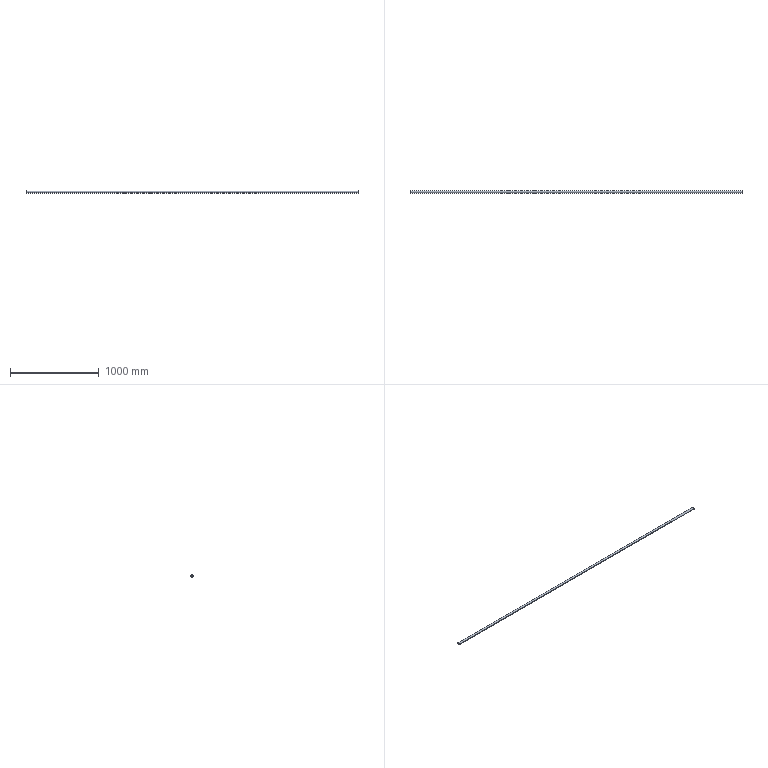Part | STEP file | 粉仓护栏栏杆2_Default<As Machined> | 1 solid | 6 faces | box 3734 x 25 x 25 mm | volume 413507 mm3 | cylinder 4 | plane 2 | commonest cylinder face diameters 22 x2 25 x2
STEP:
#1=CARTESIAN_POINT('',(0.,0.,0.));
#2=DIRECTION('',(0.,0.,1.));
#3=DIRECTION('',(1.,0.,0.));
#4=AXIS2_PLACEMENT_3D('',#1,#2,#3);
#5=CARTESIAN_POINT('',(1867.,12.5,0.));
#6=VERTEX_POINT('',#5);
#7=CARTESIAN_POINT('',(1867.,-12.5,0.));
#8=VERTEX_POINT('',#7);
#9=CARTESIAN_POINT('',(1867.,0.,0.));
#10=DIRECTION('',(1.,0.,0.));
#11=DIRECTION('',(0.,1.,0.));
#12=AXIS2_PLACEMENT_3D('',#9,#10,#11);
#13=CIRCLE('',#12,12.5);
#14=CARTESIAN_POINT('',(1867.,0.,0.));
#15=DIRECTION('',(-1.,0.,0.));
#16=DIRECTION('',(0.,-1.,0.));
#17=AXIS2_PLACEMENT_3D('',#14,#15,#16);
#18=CYLINDRICAL_SURFACE('',#17,12.5);
#19=CARTESIAN_POINT('',(3.142,0.));
#20=DIRECTION('',(-1.,0.));
#21=VECTOR('',#20,1.);
#22=LINE('',#19,#21);
#23=(GEOMETRIC_REPRESENTATION_CONTEXT(2)PARAMETRIC_REPRESENTATION_CONTEXT()REPRESENTATION_CONTEXT('',''));
#24=DEFINITIONAL_REPRESENTATION('',(#22),#23);
#25=PCURVE('',#18,#24);
#26=CARTESIAN_POINT('',(1867.,0.,0.));
#27=DIRECTION('',(1.,0.,0.));
#28=DIRECTION('',(0.,1.,0.));
#29=AXIS2_PLACEMENT_3D('',#26,#27,#28);
#30=PLANE('',#29);
#31=CARTESIAN_POINT('',(0.,0.));
#32=DIRECTION('',(1.,0.));
#33=AXIS2_PLACEMENT_2D('',#31,#32);
#34=CIRCLE('',#33,12.5);
#35=(GEOMETRIC_REPRESENTATION_CONTEXT(2)PARAMETRIC_REPRESENTATION_CONTEXT()REPRESENTATION_CONTEXT('',''));
#36=DEFINITIONAL_REPRESENTATION('',(#34),#35);
#37=PCURVE('',#30,#36);
#38=SURFACE_CURVE('',#13,(#25,#37),.PCURVE_S1.);
#39=EDGE_CURVE('',#6,#8,#38,.T.);
#40=ORIENTED_EDGE('',*,*,#39,.F.);
#41=CARTESIAN_POINT('',(-1867.,12.5,0.));
#42=VERTEX_POINT('',#41);
#43=CARTESIAN_POINT('',(1867.,12.5,0.));
#44=DIRECTION('',(-1.,0.,0.));
#45=VECTOR('',#44,1.);
#46=LINE('',#43,#45);
#47=CARTESIAN_POINT('',(3.142,0.));
#48=DIRECTION('',(0.,1.));
#49=VECTOR('',#48,1.);
#50=LINE('',#47,#49);
#51=(GEOMETRIC_REPRESENTATION_CONTEXT(2)PARAMETRIC_REPRESENTATION_CONTEXT()REPRESENTATION_CONTEXT('',''));
#52=DEFINITIONAL_REPRESENTATION('',(#50),#51);
#53=PCURVE('',#18,#52);
#54=CARTESIAN_POINT('',(1867.,0.,0.));
#55=DIRECTION('',(-1.,0.,0.));
#56=DIRECTION('',(0.,-1.,0.));
#57=AXIS2_PLACEMENT_3D('',#54,#55,#56);
#58=CYLINDRICAL_SURFACE('',#57,12.5);
#59=CARTESIAN_POINT('',(3.142,0.));
#60=DIRECTION('',(0.,1.));
#61=VECTOR('',#60,1.);
#62=LINE('',#59,#61);
#63=(GEOMETRIC_REPRESENTATION_CONTEXT(2)PARAMETRIC_REPRESENTATION_CONTEXT()REPRESENTATION_CONTEXT('',''));
#64=DEFINITIONAL_REPRESENTATION('',(#62),#63);
#65=PCURVE('',#58,#64);
#66=SURFACE_CURVE('',#46,(#53,#65),.PCURVE_S1.);
#67=EDGE_CURVE('',#6,#42,#66,.T.);
#68=ORIENTED_EDGE('',*,*,#67,.T.);
#69=CARTESIAN_POINT('',(-1867.,-12.5,0.));
#70=VERTEX_POINT('',#69);
#71=CARTESIAN_POINT('',(-1867.,0.,0.));
#72=DIRECTION('',(1.,0.,0.));
#73=DIRECTION('',(0.,1.,0.));
#74=AXIS2_PLACEMENT_3D('',#71,#72,#73);
#75=CIRCLE('',#74,12.5);
#76=CARTESIAN_POINT('',(3.142,3734.));
#77=DIRECTION('',(-1.,0.));
#78=VECTOR('',#77,1.);
#79=LINE('',#76,#78);
#80=(GEOMETRIC_REPRESENTATION_CONTEXT(2)PARAMETRIC_REPRESENTATION_CONTEXT()REPRESENTATION_CONTEXT('',''));
#81=DEFINITIONAL_REPRESENTATION('',(#79),#80);
#82=PCURVE('',#18,#81);
#83=CARTESIAN_POINT('',(-1867.,0.,0.));
#84=DIRECTION('',(1.,0.,0.));
#85=DIRECTION('',(0.,1.,0.));
#86=AXIS2_PLACEMENT_3D('',#83,#84,#85);
#87=PLANE('',#86);
#88=CARTESIAN_POINT('',(0.,0.));
#89=DIRECTION('',(1.,0.));
#90=AXIS2_PLACEMENT_2D('',#88,#89);
#91=CIRCLE('',#90,12.5);
#92=(GEOMETRIC_REPRESENTATION_CONTEXT(2)PARAMETRIC_REPRESENTATION_CONTEXT()REPRESENTATION_CONTEXT('',''));
#93=DEFINITIONAL_REPRESENTATION('',(#91),#92);
#94=PCURVE('',#87,#93);
#95=SURFACE_CURVE('',#75,(#82,#94),.PCURVE_S1.);
#96=EDGE_CURVE('',#42,#70,#95,.T.);
#97=ORIENTED_EDGE('',*,*,#96,.T.);
#98=CARTESIAN_POINT('',(1867.,-12.5,0.));
#99=DIRECTION('',(-1.,0.,0.));
#100=VECTOR('',#99,1.);
#101=LINE('',#98,#100);
#102=CARTESIAN_POINT('',(0.,0.));
#103=DIRECTION('',(0.,1.));
#104=VECTOR('',#103,1.);
#105=LINE('',#102,#104);
#106=(GEOMETRIC_REPRESENTATION_CONTEXT(2)PARAMETRIC_REPRESENTATION_CONTEXT()REPRESENTATION_CONTEXT('',''));
#107=DEFINITIONAL_REPRESENTATION('',(#105),#106);
#108=PCURVE('',#18,#107);
#109=CARTESIAN_POINT('',(6.283,0.));
#110=DIRECTION('',(0.,1.));
#111=VECTOR('',#110,1.);
#112=LINE('',#109,#111);
#113=(GEOMETRIC_REPRESENTATION_CONTEXT(2)PARAMETRIC_REPRESENTATION_CONTEXT()REPRESENTATION_CONTEXT('',''));
#114=DEFINITIONAL_REPRESENTATION('',(#112),#113);
#115=PCURVE('',#58,#114);
#116=SURFACE_CURVE('',#101,(#108,#115),.PCURVE_S1.);
#117=EDGE_CURVE('',#8,#70,#116,.T.);
#118=ORIENTED_EDGE('',*,*,#117,.F.);
#119=EDGE_LOOP('',(#40,#68,#97,#118));
#120=FACE_BOUND('',#119,.T.);
#121=ADVANCED_FACE('',(#120),#18,.T.);
#122=CARTESIAN_POINT('',(1867.,-11.,0.));
#123=VERTEX_POINT('',#122);
#124=CARTESIAN_POINT('',(-1867.,-11.,0.));
#125=VERTEX_POINT('',#124);
#126=CARTESIAN_POINT('',(1867.,-11.,0.));
#127=DIRECTION('',(-1.,0.,0.));
#128=VECTOR('',#127,1.);
#129=LINE('',#126,#128);
#130=CARTESIAN_POINT('',(1867.,0.,0.));
#131=DIRECTION('',(-1.,0.,0.));
#132=DIRECTION('',(0.,-1.,0.));
#133=AXIS2_PLACEMENT_3D('',#130,#131,#132);
#134=CYLINDRICAL_SURFACE('',#133,11.);
#135=CARTESIAN_POINT('',(6.283,0.));
#136=DIRECTION('',(0.,1.));
#137=VECTOR('',#136,1.);
#138=LINE('',#135,#137);
#139=(GEOMETRIC_REPRESENTATION_CONTEXT(2)PARAMETRIC_REPRESENTATION_CONTEXT()REPRESENTATION_CONTEXT('',''));
#140=DEFINITIONAL_REPRESENTATION('',(#138),#139);
#141=PCURVE('',#134,#140);
#142=CARTESIAN_POINT('',(1867.,0.,0.));
#143=DIRECTION('',(-1.,0.,0.));
#144=DIRECTION('',(0.,-1.,0.));
#145=AXIS2_PLACEMENT_3D('',#142,#143,#144);
#146=CYLINDRICAL_SURFACE('',#145,11.);
#147=CARTESIAN_POINT('',(0.,0.));
#148=DIRECTION('',(0.,1.));
#149=VECTOR('',#148,1.);
#150=LINE('',#147,#149);
#151=(GEOMETRIC_REPRESENTATION_CONTEXT(2)PARAMETRIC_REPRESENTATION_CONTEXT()REPRESENTATION_CONTEXT('',''));
#152=DEFINITIONAL_REPRESENTATION('',(#150),#151);
#153=PCURVE('',#146,#152);
#154=SURFACE_CURVE('',#129,(#141,#153),.PCURVE_S1.);
#155=EDGE_CURVE('',#123,#125,#154,.T.);
#156=ORIENTED_EDGE('',*,*,#155,.T.);
#157=CARTESIAN_POINT('',(-1867.,11.,0.));
#158=VERTEX_POINT('',#157);
#159=CARTESIAN_POINT('',(-1867.,0.,0.));
#160=DIRECTION('',(1.,0.,0.));
#161=DIRECTION('',(0.,1.,0.));
#162=AXIS2_PLACEMENT_3D('',#159,#160,#161);
#163=CIRCLE('',#162,11.);
#164=CARTESIAN_POINT('',(9.425,3734.));
#165=DIRECTION('',(-1.,0.));
#166=VECTOR('',#165,1.);
#167=LINE('',#164,#166);
#168=(GEOMETRIC_REPRESENTATION_CONTEXT(2)PARAMETRIC_REPRESENTATION_CONTEXT()REPRESENTATION_CONTEXT('',''));
#169=DEFINITIONAL_REPRESENTATION('',(#167),#168);
#170=PCURVE('',#134,#169);
#171=CARTESIAN_POINT('',(0.,0.));
#172=DIRECTION('',(1.,0.));
#173=AXIS2_PLACEMENT_2D('',#171,#172);
#174=CIRCLE('',#173,11.);
#175=(GEOMETRIC_REPRESENTATION_CONTEXT(2)PARAMETRIC_REPRESENTATION_CONTEXT()REPRESENTATION_CONTEXT('',''));
#176=DEFINITIONAL_REPRESENTATION('',(#174),#175);
#177=PCURVE('',#87,#176);
#178=SURFACE_CURVE('',#163,(#170,#177),.PCURVE_S1.);
#179=EDGE_CURVE('',#125,#158,#178,.T.);
#180=ORIENTED_EDGE('',*,*,#179,.T.);
#181=CARTESIAN_POINT('',(1867.,11.,0.));
#182=VERTEX_POINT('',#181);
#183=CARTESIAN_POINT('',(1867.,11.,0.));
#184=DIRECTION('',(-1.,0.,0.));
#185=VECTOR('',#184,1.);
#186=LINE('',#183,#185);
#187=CARTESIAN_POINT('',(3.142,0.));
#188=DIRECTION('',(0.,1.));
#189=VECTOR('',#188,1.);
#190=LINE('',#187,#189);
#191=(GEOMETRIC_REPRESENTATION_CONTEXT(2)PARAMETRIC_REPRESENTATION_CONTEXT()REPRESENTATION_CONTEXT('',''));
#192=DEFINITIONAL_REPRESENTATION('',(#190),#191);
#193=PCURVE('',#134,#192);
#194=CARTESIAN_POINT('',(3.142,0.));
#195=DIRECTION('',(0.,1.));
#196=VECTOR('',#195,1.);
#197=LINE('',#194,#196);
#198=(GEOMETRIC_REPRESENTATION_CONTEXT(2)PARAMETRIC_REPRESENTATION_CONTEXT()REPRESENTATION_CONTEXT('',''));
#199=DEFINITIONAL_REPRESENTATION('',(#197),#198);
#200=PCURVE('',#146,#199);
#201=SURFACE_CURVE('',#186,(#193,#200),.PCURVE_S1.);
#202=EDGE_CURVE('',#182,#158,#201,.T.);
#203=ORIENTED_EDGE('',*,*,#202,.F.);
#204=CARTESIAN_POINT('',(1867.,0.,0.));
#205=DIRECTION('',(1.,0.,0.));
#206=DIRECTION('',(0.,1.,0.));
#207=AXIS2_PLACEMENT_3D('',#204,#205,#206);
#208=CIRCLE('',#207,11.);
#209=CARTESIAN_POINT('',(9.425,0.));
#210=DIRECTION('',(-1.,0.));
#211=VECTOR('',#210,1.);
#212=LINE('',#209,#211);
#213=(GEOMETRIC_REPRESENTATION_CONTEXT(2)PARAMETRIC_REPRESENTATION_CONTEXT()REPRESENTATION_CONTEXT('',''));
#214=DEFINITIONAL_REPRESENTATION('',(#212),#213);
#215=PCURVE('',#134,#214);
#216=CARTESIAN_POINT('',(0.,0.));
#217=DIRECTION('',(1.,0.));
#218=AXIS2_PLACEMENT_2D('',#216,#217);
#219=CIRCLE('',#218,11.);
#220=(GEOMETRIC_REPRESENTATION_CONTEXT(2)PARAMETRIC_REPRESENTATION_CONTEXT()REPRESENTATION_CONTEXT('',''));
#221=DEFINITIONAL_REPRESENTATION('',(#219),#220);
#222=PCURVE('',#30,#221);
#223=SURFACE_CURVE('',#208,(#215,#222),.PCURVE_S1.);
#224=EDGE_CURVE('',#123,#182,#223,.T.);
#225=ORIENTED_EDGE('',*,*,#224,.F.);
#226=EDGE_LOOP('',(#156,#180,#203,#225));
#227=FACE_BOUND('',#226,.F.);
#228=ADVANCED_FACE('',(#227),#134,.F.);
#229=CARTESIAN_POINT('',(-1867.,0.,0.));
#230=DIRECTION('',(1.,0.,0.));
#231=DIRECTION('',(0.,1.,0.));
#232=AXIS2_PLACEMENT_3D('',#229,#230,#231);
#233=CIRCLE('',#232,11.);
#234=CARTESIAN_POINT('',(3.142,3734.));
#235=DIRECTION('',(-1.,0.));
#236=VECTOR('',#235,1.);
#237=LINE('',#234,#236);
#238=(GEOMETRIC_REPRESENTATION_CONTEXT(2)PARAMETRIC_REPRESENTATION_CONTEXT()REPRESENTATION_CONTEXT('',''));
#239=DEFINITIONAL_REPRESENTATION('',(#237),#238);
#240=PCURVE('',#146,#239);
#241=CARTESIAN_POINT('',(0.,0.));
#242=DIRECTION('',(1.,0.));
#243=AXIS2_PLACEMENT_2D('',#241,#242);
#244=CIRCLE('',#243,11.);
#245=(GEOMETRIC_REPRESENTATION_CONTEXT(2)PARAMETRIC_REPRESENTATION_CONTEXT()REPRESENTATION_CONTEXT('',''));
#246=DEFINITIONAL_REPRESENTATION('',(#244),#245);
#247=PCURVE('',#87,#246);
#248=SURFACE_CURVE('',#233,(#240,#247),.PCURVE_S1.);
#249=EDGE_CURVE('',#158,#125,#248,.T.);
#250=ORIENTED_EDGE('',*,*,#249,.T.);
#251=ORIENTED_EDGE('',*,*,#155,.F.);
#252=CARTESIAN_POINT('',(1867.,0.,0.));
#253=DIRECTION('',(1.,0.,0.));
#254=DIRECTION('',(0.,1.,0.));
#255=AXIS2_PLACEMENT_3D('',#252,#253,#254);
#256=CIRCLE('',#255,11.);
#257=CARTESIAN_POINT('',(3.142,0.));
#258=DIRECTION('',(-1.,0.));
#259=VECTOR('',#258,1.);
#260=LINE('',#257,#259);
#261=(GEOMETRIC_REPRESENTATION_CONTEXT(2)PARAMETRIC_REPRESENTATION_CONTEXT()REPRESENTATION_CONTEXT('',''));
#262=DEFINITIONAL_REPRESENTATION('',(#260),#261);
#263=PCURVE('',#146,#262);
#264=CARTESIAN_POINT('',(0.,0.));
#265=DIRECTION('',(1.,0.));
#266=AXIS2_PLACEMENT_2D('',#264,#265);
#267=CIRCLE('',#266,11.);
#268=(GEOMETRIC_REPRESENTATION_CONTEXT(2)PARAMETRIC_REPRESENTATION_CONTEXT()REPRESENTATION_CONTEXT('',''));
#269=DEFINITIONAL_REPRESENTATION('',(#267),#268);
#270=PCURVE('',#30,#269);
#271=SURFACE_CURVE('',#256,(#263,#270),.PCURVE_S1.);
#272=EDGE_CURVE('',#182,#123,#271,.T.);
#273=ORIENTED_EDGE('',*,*,#272,.F.);
#274=ORIENTED_EDGE('',*,*,#202,.T.);
#275=EDGE_LOOP('',(#250,#251,#273,#274));
#276=FACE_BOUND('',#275,.F.);
#277=ADVANCED_FACE('',(#276),#146,.F.);
#278=ORIENTED_EDGE('',*,*,#67,.F.);
#279=CARTESIAN_POINT('',(1867.,0.,0.));
#280=DIRECTION('',(1.,0.,0.));
#281=DIRECTION('',(0.,1.,0.));
#282=AXIS2_PLACEMENT_3D('',#279,#280,#281);
#283=CIRCLE('',#282,12.5);
#284=CARTESIAN_POINT('',(9.425,0.));
#285=DIRECTION('',(-1.,0.));
#286=VECTOR('',#285,1.);
#287=LINE('',#284,#286);
#288=(GEOMETRIC_REPRESENTATION_CONTEXT(2)PARAMETRIC_REPRESENTATION_CONTEXT()REPRESENTATION_CONTEXT('',''));
#289=DEFINITIONAL_REPRESENTATION('',(#287),#288);
#290=PCURVE('',#58,#289);
#291=CARTESIAN_POINT('',(0.,0.));
#292=DIRECTION('',(1.,0.));
#293=AXIS2_PLACEMENT_2D('',#291,#292);
#294=CIRCLE('',#293,12.5);
#295=(GEOMETRIC_REPRESENTATION_CONTEXT(2)PARAMETRIC_REPRESENTATION_CONTEXT()REPRESENTATION_CONTEXT('',''));
#296=DEFINITIONAL_REPRESENTATION('',(#294),#295);
#297=PCURVE('',#30,#296);
#298=SURFACE_CURVE('',#283,(#290,#297),.PCURVE_S1.);
#299=EDGE_CURVE('',#8,#6,#298,.T.);
#300=ORIENTED_EDGE('',*,*,#299,.F.);
#301=ORIENTED_EDGE('',*,*,#117,.T.);
#302=CARTESIAN_POINT('',(-1867.,0.,0.));
#303=DIRECTION('',(1.,0.,0.));
#304=DIRECTION('',(0.,1.,0.));
#305=AXIS2_PLACEMENT_3D('',#302,#303,#304);
#306=CIRCLE('',#305,12.5);
#307=CARTESIAN_POINT('',(9.425,3734.));
#308=DIRECTION('',(-1.,0.));
#309=VECTOR('',#308,1.);
#310=LINE('',#307,#309);
#311=(GEOMETRIC_REPRESENTATION_CONTEXT(2)PARAMETRIC_REPRESENTATION_CONTEXT()REPRESENTATION_CONTEXT('',''));
#312=DEFINITIONAL_REPRESENTATION('',(#310),#311);
#313=PCURVE('',#58,#312);
#314=CARTESIAN_POINT('',(0.,0.));
#315=DIRECTION('',(1.,0.));
#316=AXIS2_PLACEMENT_2D('',#314,#315);
#317=CIRCLE('',#316,12.5);
#318=(GEOMETRIC_REPRESENTATION_CONTEXT(2)PARAMETRIC_REPRESENTATION_CONTEXT()REPRESENTATION_CONTEXT('',''));
#319=DEFINITIONAL_REPRESENTATION('',(#317),#318);
#320=PCURVE('',#87,#319);
#321=SURFACE_CURVE('',#306,(#313,#320),.PCURVE_S1.);
#322=EDGE_CURVE('',#70,#42,#321,.T.);
#323=ORIENTED_EDGE('',*,*,#322,.T.);
#324=EDGE_LOOP('',(#278,#300,#301,#323));
#325=FACE_BOUND('',#324,.T.);
#326=ADVANCED_FACE('',(#325),#58,.T.);
#327=ORIENTED_EDGE('',*,*,#224,.F.);
#328=ORIENTED_EDGE('',*,*,#272,.F.);
#329=EDGE_LOOP('',(#327,#328));
#330=FACE_BOUND('',#329,.T.);
#331=ORIENTED_EDGE('',*,*,#299,.T.);
#332=ORIENTED_EDGE('',*,*,#39,.T.);
#333=EDGE_LOOP('',(#331,#332));
#334=FACE_BOUND('',#333,.T.);
#335=ADVANCED_FACE('',(#330,#334),#30,.T.);
#336=ORIENTED_EDGE('',*,*,#179,.T.);
#337=ORIENTED_EDGE('',*,*,#249,.T.);
#338=EDGE_LOOP('',(#336,#337));
#339=FACE_BOUND('',#338,.T.);
#340=ORIENTED_EDGE('',*,*,#322,.F.);
#341=ORIENTED_EDGE('',*,*,#96,.F.);
#342=EDGE_LOOP('',(#340,#341));
#343=FACE_BOUND('',#342,.T.);
#344=ADVANCED_FACE('',(#339,#343),#87,.F.);
#345=CLOSED_SHELL('',(#121,#228,#277,#326,#335,#344));
#346=MANIFOLD_SOLID_BREP('',#345);
#347=(LENGTH_UNIT()NAMED_UNIT(*)SI_UNIT(.MILLI.,.METRE.));
#348=UNCERTAINTY_MEASURE_WITH_UNIT(LENGTH_MEASURE(0.0000001),#347,'','');
#349=(NAMED_UNIT(*)PLANE_ANGLE_UNIT()SI_UNIT($,.RADIAN.));
#350=(NAMED_UNIT(*)SI_UNIT($,.STERADIAN.)SOLID_ANGLE_UNIT());
#351=(GEOMETRIC_REPRESENTATION_CONTEXT(3)GLOBAL_UNCERTAINTY_ASSIGNED_CONTEXT((#348))GLOBAL_UNIT_ASSIGNED_CONTEXT((#347,#349,#350))REPRESENTATION_CONTEXT('',''));
#352=ADVANCED_BREP_SHAPE_REPRESENTATION('',(#4,#346),#351);